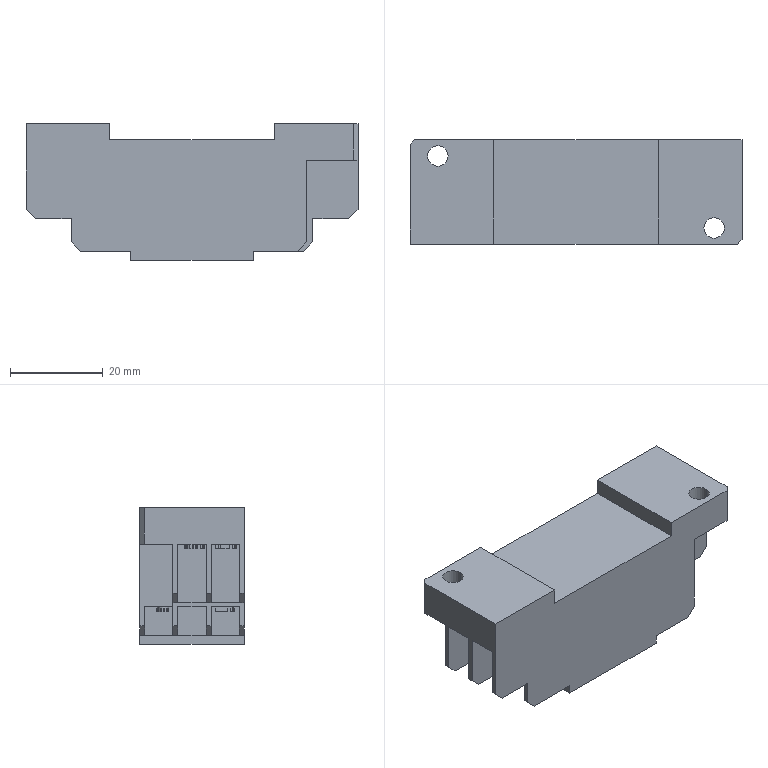Part | STEP file | Fixing bracket 1 | 1 solid | 413 faces | box 71.5 x 22.5 x 29.5 mm | volume 31610 mm3 | plane 409 | cylinder 4 | commonest cylinder face diameters 4.4 x4